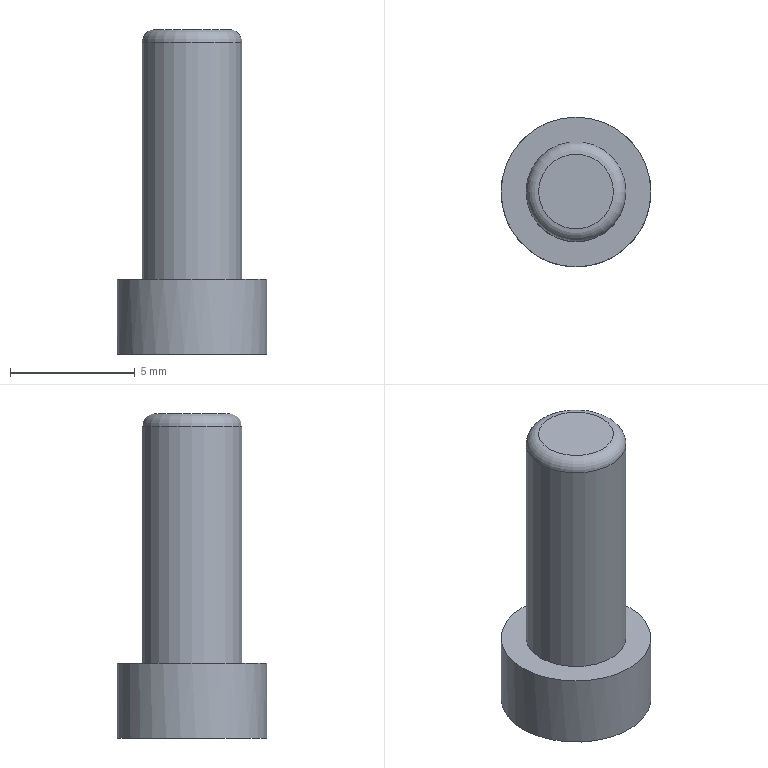Part | STEP file | gslz 2016.10.28-6_id502_x_t | 1 solid | 6 faces | box 6 x 6 x 13 mm | volume 209.85 mm3 | plane 3 | cylinder 2 | torus 1 | commonest cylinder face diameters 4 x1 6 x1
STEP:
#1=CARTESIAN_POINT('',(-81.95,192.,49.));
#2=VERTEX_POINT('',#1);
#3=CARTESIAN_POINT('',(-81.95,189.,49.));
#4=DIRECTION('',(0.,0.,-1.));
#5=DIRECTION('',(0.,1.,0.));
#6=AXIS2_PLACEMENT_3D('',#3,#4,#5);
#7=CIRCLE('',#6,3.);
#8=EDGE_CURVE('',#2,#2,#7,.T.);
#9=ORIENTED_EDGE('',*,*,#8,.T.);
#10=EDGE_LOOP('',(#9));
#11=FACE_OUTER_BOUND('',#10,.T.);
#12=CARTESIAN_POINT('',(-26.511,233.829,49.));
#13=DIRECTION('',(0.,0.,-1.));
#14=DIRECTION('',(-1.,0.,0.));
#15=AXIS2_PLACEMENT_3D('',#12,#13,#14);
#16=PLANE('',#15);
#17=ADVANCED_FACE('',(#11),#16,.T.);
#18=CARTESIAN_POINT('',(-79.95,189.,52.));
#19=VERTEX_POINT('',#18);
#20=CARTESIAN_POINT('',(-81.95,189.,52.));
#21=DIRECTION('',(0.,0.,-1.));
#22=DIRECTION('',(1.,0.,0.));
#23=AXIS2_PLACEMENT_3D('',#20,#21,#22);
#24=CIRCLE('',#23,2.);
#25=EDGE_CURVE('',#19,#19,#24,.T.);
#26=ORIENTED_EDGE('',*,*,#25,.T.);
#27=EDGE_LOOP('',(#26));
#28=FACE_BOUND('',#27,.T.);
#29=CARTESIAN_POINT('',(-78.95,189.,52.));
#30=VERTEX_POINT('',#29);
#31=CARTESIAN_POINT('',(-81.95,189.,52.));
#32=DIRECTION('',(0.,0.,1.));
#33=DIRECTION('',(1.,0.,0.));
#34=AXIS2_PLACEMENT_3D('',#31,#32,#33);
#35=CIRCLE('',#34,3.);
#36=EDGE_CURVE('',#30,#30,#35,.T.);
#37=ORIENTED_EDGE('',*,*,#36,.T.);
#38=EDGE_LOOP('',(#37));
#39=FACE_BOUND('',#38,.T.);
#40=CARTESIAN_POINT('',(-81.95,189.,52.));
#41=DIRECTION('',(0.,0.,1.));
#42=DIRECTION('',(1.,0.,0.));
#43=AXIS2_PLACEMENT_3D('',#40,#41,#42);
#44=PLANE('',#43);
#45=ADVANCED_FACE('',(#28,#39),#44,.T.);
#46=ORIENTED_EDGE('',*,*,#8,.F.);
#47=EDGE_LOOP('',(#46));
#48=FACE_BOUND('',#47,.T.);
#49=ORIENTED_EDGE('',*,*,#36,.F.);
#50=EDGE_LOOP('',(#49));
#51=FACE_BOUND('',#50,.T.);
#52=CARTESIAN_POINT('',(-81.95,189.,70.));
#53=DIRECTION('',(0.,0.,-1.));
#54=DIRECTION('',(-1.,0.,0.));
#55=AXIS2_PLACEMENT_3D('',#52,#53,#54);
#56=CYLINDRICAL_SURFACE('',#55,3.);
#57=ADVANCED_FACE('',(#48,#51),#56,.T.);
#58=CARTESIAN_POINT('',(-80.45,189.,62.));
#59=VERTEX_POINT('',#58);
#60=CARTESIAN_POINT('',(-81.95,189.,62.));
#61=DIRECTION('',(0.,0.,1.));
#62=DIRECTION('',(1.,0.,0.));
#63=AXIS2_PLACEMENT_3D('',#60,#61,#62);
#64=CIRCLE('',#63,1.5);
#65=EDGE_CURVE('',#59,#59,#64,.T.);
#66=ORIENTED_EDGE('',*,*,#65,.T.);
#67=EDGE_LOOP('',(#66));
#68=FACE_OUTER_BOUND('',#67,.T.);
#69=CARTESIAN_POINT('',(-81.95,189.,62.));
#70=DIRECTION('',(0.,0.,1.));
#71=DIRECTION('',(1.,0.,0.));
#72=AXIS2_PLACEMENT_3D('',#69,#70,#71);
#73=PLANE('',#72);
#74=ADVANCED_FACE('',(#68),#73,.T.);
#75=CARTESIAN_POINT('',(-79.95,189.,61.5));
#76=VERTEX_POINT('',#75);
#77=CARTESIAN_POINT('',(-81.95,189.,61.5));
#78=DIRECTION('',(0.,0.,-1.));
#79=DIRECTION('',(1.,0.,0.));
#80=AXIS2_PLACEMENT_3D('',#77,#78,#79);
#81=CIRCLE('',#80,2.);
#82=EDGE_CURVE('',#76,#76,#81,.T.);
#83=ORIENTED_EDGE('',*,*,#82,.T.);
#84=EDGE_LOOP('',(#83));
#85=FACE_BOUND('',#84,.T.);
#86=ORIENTED_EDGE('',*,*,#25,.F.);
#87=EDGE_LOOP('',(#86));
#88=FACE_BOUND('',#87,.T.);
#89=CARTESIAN_POINT('',(-81.95,189.,52.));
#90=DIRECTION('',(0.,0.,1.));
#91=DIRECTION('',(1.,0.,0.));
#92=AXIS2_PLACEMENT_3D('',#89,#90,#91);
#93=CYLINDRICAL_SURFACE('',#92,2.);
#94=ADVANCED_FACE('',(#85,#88),#93,.T.);
#95=ORIENTED_EDGE('',*,*,#82,.F.);
#96=EDGE_LOOP('',(#95));
#97=FACE_BOUND('',#96,.T.);
#98=ORIENTED_EDGE('',*,*,#65,.F.);
#99=EDGE_LOOP('',(#98));
#100=FACE_BOUND('',#99,.T.);
#101=CARTESIAN_POINT('',(-81.95,189.,61.5));
#102=DIRECTION('',(0.,0.,1.));
#103=DIRECTION('',(-1.,0.,0.));
#104=AXIS2_PLACEMENT_3D('',#101,#102,#103);
#105=TOROIDAL_SURFACE('',#104,1.5,0.5);
#106=ADVANCED_FACE('',(#97,#100),#105,.T.);
#107=CLOSED_SHELL('',(#17,#45,#57,#74,#94,#106));
#108=MANIFOLD_SOLID_BREP('',#107);
#109=(LENGTH_UNIT()NAMED_UNIT(*)SI_UNIT(.MILLI.,.METRE.));
#110=UNCERTAINTY_MEASURE_WITH_UNIT(LENGTH_MEASURE(0.00002),#109,'','');
#111=(NAMED_UNIT(*)PLANE_ANGLE_UNIT()SI_UNIT($,.RADIAN.));
#112=PLANE_ANGLE_MEASURE_WITH_UNIT(PLANE_ANGLE_MEASURE(0.01745),#111);
#113=DIMENSIONAL_EXPONENTS(0.,0.,0.,0.,0.,0.,0.);
#114=(CONVERSION_BASED_UNIT('DEGREE',#112)NAMED_UNIT(#113)PLANE_ANGLE_UNIT());
#115=(NAMED_UNIT(*)SI_UNIT($,.STERADIAN.)SOLID_ANGLE_UNIT());
#116=(GEOMETRIC_REPRESENTATION_CONTEXT(3)GLOBAL_UNCERTAINTY_ASSIGNED_CONTEXT((#110))GLOBAL_UNIT_ASSIGNED_CONTEXT((#109,#114,#115))REPRESENTATION_CONTEXT('',''));
#117=ADVANCED_BREP_SHAPE_REPRESENTATION('',(#108),#116);